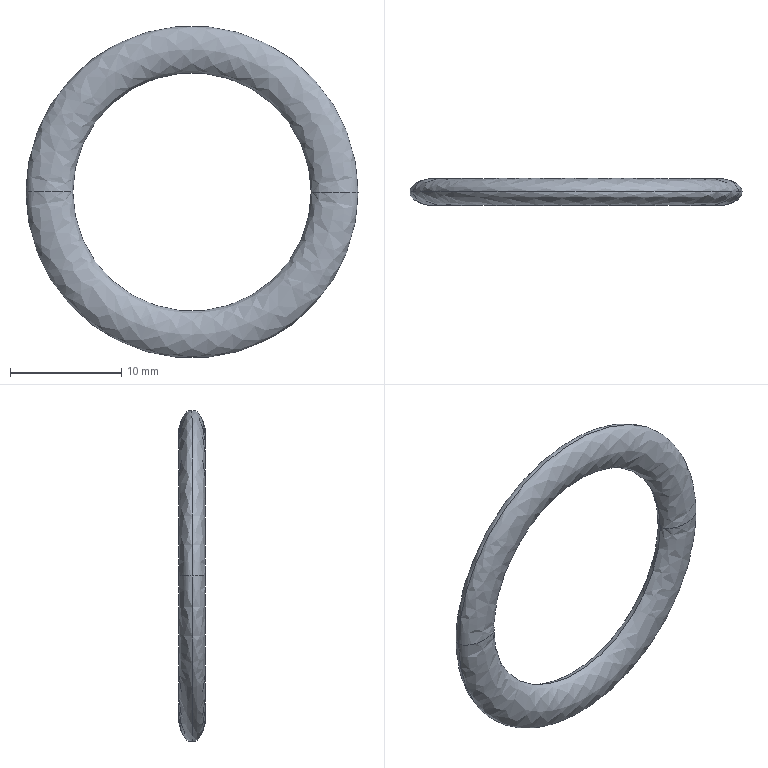Part | SolidWorks | features Revolution 2 | 1 solid | 4 faces | box 29.8 x 2.4 x 29.8 mm | volume 636.708 mm3 | spline 4
STEP:
#1=CARTESIAN_POINT('',(4.2,1.2,0.));
#2=VERTEX_POINT('',#1);
#3=CARTESIAN_POINT('',(25.6,1.2,0.));
#4=VERTEX_POINT('',#3);
#5=CARTESIAN_POINT('',(14.9,1.2,0.));
#6=DIRECTION('',(0.,-1.,0.));
#7=DIRECTION('',(-1.,0.,0.));
#8=AXIS2_PLACEMENT_3D('',#5,#6,#7);
#9=CIRCLE('',#8,10.7);
#10=EDGE_CURVE('',#2,#4,#9,.T.);
#11=ORIENTED_EDGE('',*,*,#10,.T.);
#12=CARTESIAN_POINT('',(29.8,1.2,0.));
#13=VERTEX_POINT('',#12);
#14=CARTESIAN_POINT('',(25.6,1.2,0.));
#15=CARTESIAN_POINT('',(25.6,3.6,0.));
#16=CARTESIAN_POINT('',(29.8,3.6,0.));
#17=CARTESIAN_POINT('',(29.8,1.2,0.));
#18=(BOUNDED_CURVE()B_SPLINE_CURVE(3,(#14,#15,#16,#17),.UNSPECIFIED.,.F.,.T.)B_SPLINE_CURVE_WITH_KNOTS((4,4),(0.,3.142),.UNSPECIFIED.)CURVE()GEOMETRIC_REPRESENTATION_ITEM()RATIONAL_B_SPLINE_CURVE((1.,0.3333,0.3333,1.))REPRESENTATION_ITEM(''));
#19=EDGE_CURVE('',#4,#13,#18,.T.);
#20=ORIENTED_EDGE('',*,*,#19,.T.);
#21=CARTESIAN_POINT('',(0.,1.2,0.));
#22=VERTEX_POINT('',#21);
#23=CARTESIAN_POINT('',(14.9,1.2,0.));
#24=DIRECTION('',(0.,-1.,0.));
#25=DIRECTION('',(-1.,0.,0.));
#26=AXIS2_PLACEMENT_3D('',#23,#24,#25);
#27=CIRCLE('',#26,14.9);
#28=EDGE_CURVE('',#22,#13,#27,.T.);
#29=ORIENTED_EDGE('',*,*,#28,.F.);
#30=CARTESIAN_POINT('',(4.2,1.2,0.));
#31=CARTESIAN_POINT('',(4.2,3.6,0.));
#32=CARTESIAN_POINT('',(0.,3.6,0.));
#33=CARTESIAN_POINT('',(0.,1.2,0.));
#34=(BOUNDED_CURVE()B_SPLINE_CURVE(3,(#30,#31,#32,#33),.UNSPECIFIED.,.F.,.F.)B_SPLINE_CURVE_WITH_KNOTS((4,4),(0.,3.142),.UNSPECIFIED.)CURVE()GEOMETRIC_REPRESENTATION_ITEM()RATIONAL_B_SPLINE_CURVE((1.,0.3333,0.3333,1.))REPRESENTATION_ITEM(''));
#35=EDGE_CURVE('',#2,#22,#34,.T.);
#36=ORIENTED_EDGE('',*,*,#35,.F.);
#37=EDGE_LOOP('',(#11,#20,#29,#36));
#38=FACE_OUTER_BOUND('',#37,.T.);
#39=CARTESIAN_POINT('',(4.2,1.2,0.));
#40=CARTESIAN_POINT('',(4.2,1.2,-21.4));
#41=CARTESIAN_POINT('',(25.6,1.2,-21.4));
#42=CARTESIAN_POINT('',(25.6,1.2,0.));
#43=CARTESIAN_POINT('',(4.2,3.6,0.));
#44=CARTESIAN_POINT('',(4.2,3.6,-21.4));
#45=CARTESIAN_POINT('',(25.6,3.6,-21.4));
#46=CARTESIAN_POINT('',(25.6,3.6,0.));
#47=CARTESIAN_POINT('',(0.,3.6,0.));
#48=CARTESIAN_POINT('',(0.,3.6,-29.8));
#49=CARTESIAN_POINT('',(29.8,3.6,-29.8));
#50=CARTESIAN_POINT('',(29.8,3.6,0.));
#51=CARTESIAN_POINT('',(0.,1.2,0.));
#52=CARTESIAN_POINT('',(0.,1.2,-29.8));
#53=CARTESIAN_POINT('',(29.8,1.2,-29.8));
#54=CARTESIAN_POINT('',(29.8,1.2,0.));
#55=(BOUNDED_SURFACE()B_SPLINE_SURFACE(3,3,((#39,#40,#41,#42),(#43,#44,#45,#46),(#47,#48,#49,#50),(#51,#52,#53,#54)),.UNSPECIFIED.,.F.,.F.,.F.)B_SPLINE_SURFACE_WITH_KNOTS((4,4),(4,4),(0.,1.),(0.,1.),.UNSPECIFIED.)GEOMETRIC_REPRESENTATION_ITEM()RATIONAL_B_SPLINE_SURFACE(((1.,0.3333,0.3333,1.),(0.3333,0.1111,0.1111,0.3333),(0.3333,0.1111,0.1111,0.3333),(1.,0.3333,0.3333,1.)))REPRESENTATION_ITEM('')SURFACE());
#56=ADVANCED_FACE('',(#38),#55,.F.);
#57=ORIENTED_EDGE('',*,*,#28,.T.);
#58=CARTESIAN_POINT('',(29.8,1.2,0.));
#59=CARTESIAN_POINT('',(29.8,-1.2,0.));
#60=CARTESIAN_POINT('',(25.6,-1.2,0.));
#61=CARTESIAN_POINT('',(25.6,1.2,0.));
#62=(BOUNDED_CURVE()B_SPLINE_CURVE(3,(#58,#59,#60,#61),.UNSPECIFIED.,.F.,.F.)B_SPLINE_CURVE_WITH_KNOTS((4,4),(3.142,6.283),.UNSPECIFIED.)CURVE()GEOMETRIC_REPRESENTATION_ITEM()RATIONAL_B_SPLINE_CURVE((1.,0.3333,0.3333,1.))REPRESENTATION_ITEM(''));
#63=EDGE_CURVE('',#13,#4,#62,.T.);
#64=ORIENTED_EDGE('',*,*,#63,.T.);
#65=ORIENTED_EDGE('',*,*,#10,.F.);
#66=CARTESIAN_POINT('',(0.,1.2,0.));
#67=CARTESIAN_POINT('',(0.,-1.2,0.));
#68=CARTESIAN_POINT('',(4.2,-1.2,0.));
#69=CARTESIAN_POINT('',(4.2,1.2,0.));
#70=(BOUNDED_CURVE()B_SPLINE_CURVE(3,(#66,#67,#68,#69),.UNSPECIFIED.,.F.,.T.)B_SPLINE_CURVE_WITH_KNOTS((4,4),(3.142,6.283),.UNSPECIFIED.)CURVE()GEOMETRIC_REPRESENTATION_ITEM()RATIONAL_B_SPLINE_CURVE((1.,0.3333,0.3333,1.))REPRESENTATION_ITEM(''));
#71=EDGE_CURVE('',#22,#2,#70,.T.);
#72=ORIENTED_EDGE('',*,*,#71,.F.);
#73=EDGE_LOOP('',(#57,#64,#65,#72));
#74=FACE_OUTER_BOUND('',#73,.T.);
#75=CARTESIAN_POINT('',(0.,1.2,0.));
#76=CARTESIAN_POINT('',(0.,1.2,-29.8));
#77=CARTESIAN_POINT('',(29.8,1.2,-29.8));
#78=CARTESIAN_POINT('',(29.8,1.2,0.));
#79=CARTESIAN_POINT('',(0.,-1.2,0.));
#80=CARTESIAN_POINT('',(0.,-1.2,-29.8));
#81=CARTESIAN_POINT('',(29.8,-1.2,-29.8));
#82=CARTESIAN_POINT('',(29.8,-1.2,0.));
#83=CARTESIAN_POINT('',(4.2,-1.2,0.));
#84=CARTESIAN_POINT('',(4.2,-1.2,-21.4));
#85=CARTESIAN_POINT('',(25.6,-1.2,-21.4));
#86=CARTESIAN_POINT('',(25.6,-1.2,0.));
#87=CARTESIAN_POINT('',(4.2,1.2,0.));
#88=CARTESIAN_POINT('',(4.2,1.2,-21.4));
#89=CARTESIAN_POINT('',(25.6,1.2,-21.4));
#90=CARTESIAN_POINT('',(25.6,1.2,0.));
#91=(BOUNDED_SURFACE()B_SPLINE_SURFACE(3,3,((#75,#76,#77,#78),(#79,#80,#81,#82),(#83,#84,#85,#86),(#87,#88,#89,#90)),.UNSPECIFIED.,.F.,.F.,.F.)B_SPLINE_SURFACE_WITH_KNOTS((4,4),(4,4),(0.,1.),(0.,1.),.UNSPECIFIED.)GEOMETRIC_REPRESENTATION_ITEM()RATIONAL_B_SPLINE_SURFACE(((1.,0.3333,0.3333,1.),(0.3333,0.1111,0.1111,0.3333),(0.3333,0.1111,0.1111,0.3333),(1.,0.3333,0.3333,1.)))REPRESENTATION_ITEM('')SURFACE());
#92=ADVANCED_FACE('',(#74),#91,.F.);
#93=ORIENTED_EDGE('',*,*,#63,.F.);
#94=CARTESIAN_POINT('',(14.9,1.2,0.));
#95=DIRECTION('',(0.,-1.,0.));
#96=DIRECTION('',(-1.,0.,0.));
#97=AXIS2_PLACEMENT_3D('',#94,#95,#96);
#98=CIRCLE('',#97,14.9);
#99=EDGE_CURVE('',#13,#22,#98,.T.);
#100=ORIENTED_EDGE('',*,*,#99,.T.);
#101=ORIENTED_EDGE('',*,*,#71,.T.);
#102=CARTESIAN_POINT('',(14.9,1.2,0.));
#103=DIRECTION('',(0.,-1.,0.));
#104=DIRECTION('',(-1.,0.,0.));
#105=AXIS2_PLACEMENT_3D('',#102,#103,#104);
#106=CIRCLE('',#105,10.7);
#107=EDGE_CURVE('',#4,#2,#106,.T.);
#108=ORIENTED_EDGE('',*,*,#107,.F.);
#109=EDGE_LOOP('',(#93,#100,#101,#108));
#110=FACE_OUTER_BOUND('',#109,.T.);
#111=CARTESIAN_POINT('',(29.8,1.2,0.));
#112=CARTESIAN_POINT('',(29.8,1.2,29.8));
#113=CARTESIAN_POINT('',(0.,1.2,29.8));
#114=CARTESIAN_POINT('',(0.,1.2,0.));
#115=CARTESIAN_POINT('',(29.8,-1.2,0.));
#116=CARTESIAN_POINT('',(29.8,-1.2,29.8));
#117=CARTESIAN_POINT('',(0.,-1.2,29.8));
#118=CARTESIAN_POINT('',(0.,-1.2,0.));
#119=CARTESIAN_POINT('',(25.6,-1.2,0.));
#120=CARTESIAN_POINT('',(25.6,-1.2,21.4));
#121=CARTESIAN_POINT('',(4.2,-1.2,21.4));
#122=CARTESIAN_POINT('',(4.2,-1.2,0.));
#123=CARTESIAN_POINT('',(25.6,1.2,0.));
#124=CARTESIAN_POINT('',(25.6,1.2,21.4));
#125=CARTESIAN_POINT('',(4.2,1.2,21.4));
#126=CARTESIAN_POINT('',(4.2,1.2,0.));
#127=(BOUNDED_SURFACE()B_SPLINE_SURFACE(3,3,((#111,#112,#113,#114),(#115,#116,#117,#118),(#119,#120,#121,#122),(#123,#124,#125,#126)),.UNSPECIFIED.,.F.,.F.,.F.)B_SPLINE_SURFACE_WITH_KNOTS((4,4),(4,4),(0.,1.),(0.,1.),.UNSPECIFIED.)GEOMETRIC_REPRESENTATION_ITEM()RATIONAL_B_SPLINE_SURFACE(((1.,0.3333,0.3333,1.),(0.3333,0.1111,0.1111,0.3333),(0.3333,0.1111,0.1111,0.3333),(1.,0.3333,0.3333,1.)))REPRESENTATION_ITEM('')SURFACE());
#128=ADVANCED_FACE('',(#110),#127,.F.);
#129=ORIENTED_EDGE('',*,*,#19,.F.);
#130=ORIENTED_EDGE('',*,*,#107,.T.);
#131=ORIENTED_EDGE('',*,*,#35,.T.);
#132=ORIENTED_EDGE('',*,*,#99,.F.);
#133=EDGE_LOOP('',(#129,#130,#131,#132));
#134=FACE_OUTER_BOUND('',#133,.T.);
#135=CARTESIAN_POINT('',(25.6,1.2,0.));
#136=CARTESIAN_POINT('',(25.6,1.2,21.4));
#137=CARTESIAN_POINT('',(4.2,1.2,21.4));
#138=CARTESIAN_POINT('',(4.2,1.2,0.));
#139=CARTESIAN_POINT('',(25.6,3.6,0.));
#140=CARTESIAN_POINT('',(25.6,3.6,21.4));
#141=CARTESIAN_POINT('',(4.2,3.6,21.4));
#142=CARTESIAN_POINT('',(4.2,3.6,0.));
#143=CARTESIAN_POINT('',(29.8,3.6,0.));
#144=CARTESIAN_POINT('',(29.8,3.6,29.8));
#145=CARTESIAN_POINT('',(0.,3.6,29.8));
#146=CARTESIAN_POINT('',(0.,3.6,0.));
#147=CARTESIAN_POINT('',(29.8,1.2,0.));
#148=CARTESIAN_POINT('',(29.8,1.2,29.8));
#149=CARTESIAN_POINT('',(0.,1.2,29.8));
#150=CARTESIAN_POINT('',(0.,1.2,0.));
#151=(BOUNDED_SURFACE()B_SPLINE_SURFACE(3,3,((#135,#136,#137,#138),(#139,#140,#141,#142),(#143,#144,#145,#146),(#147,#148,#149,#150)),.UNSPECIFIED.,.F.,.F.,.F.)B_SPLINE_SURFACE_WITH_KNOTS((4,4),(4,4),(0.,1.),(0.,1.),.UNSPECIFIED.)GEOMETRIC_REPRESENTATION_ITEM()RATIONAL_B_SPLINE_SURFACE(((1.,0.3333,0.3333,1.),(0.3333,0.1111,0.1111,0.3333),(0.3333,0.1111,0.1111,0.3333),(1.,0.3333,0.3333,1.)))REPRESENTATION_ITEM('')SURFACE());
#152=ADVANCED_FACE('',(#134),#151,.F.);
#153=CLOSED_SHELL('',(#56,#92,#128,#152));
#154=MANIFOLD_SOLID_BREP('',#153);
#155=CARTESIAN_POINT('',(0.,0.,0.));
#156=DIRECTION('',(0.,0.,1.));
#157=DIRECTION('',(1.,0.,0.));
#158=AXIS2_PLACEMENT_3D('',#155,#156,#157);
#159=(LENGTH_UNIT()NAMED_UNIT(*)SI_UNIT(.MILLI.,.METRE.));
#160=UNCERTAINTY_MEASURE_WITH_UNIT(LENGTH_MEASURE(0.00001),#159,'','');
#161=(NAMED_UNIT(*)PLANE_ANGLE_UNIT()SI_UNIT($,.RADIAN.));
#162=(NAMED_UNIT(*)SI_UNIT($,.STERADIAN.)SOLID_ANGLE_UNIT());
#163=(GEOMETRIC_REPRESENTATION_CONTEXT(3)GLOBAL_UNCERTAINTY_ASSIGNED_CONTEXT((#160))GLOBAL_UNIT_ASSIGNED_CONTEXT((#159,#161,#162))REPRESENTATION_CONTEXT('',''));
#164=ADVANCED_BREP_SHAPE_REPRESENTATION('',(#154,#158),#163);